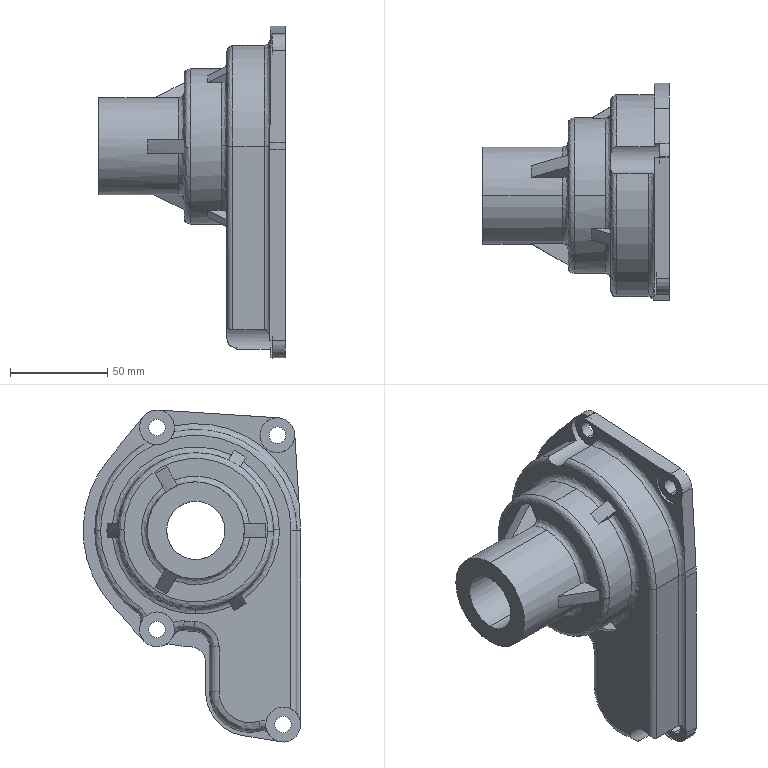Part | SolidWorks | features BaseBody 1 | 1 solid | 113 faces | box 96 x 112 x 171 mm | volume 309301 mm3 | cylinder 51 | plane 34 | spline 22 | cone 6 | commonest cylinder face diameters 18 x13 8.5 x8 10 x6 6 x4 104 x3 16 x2